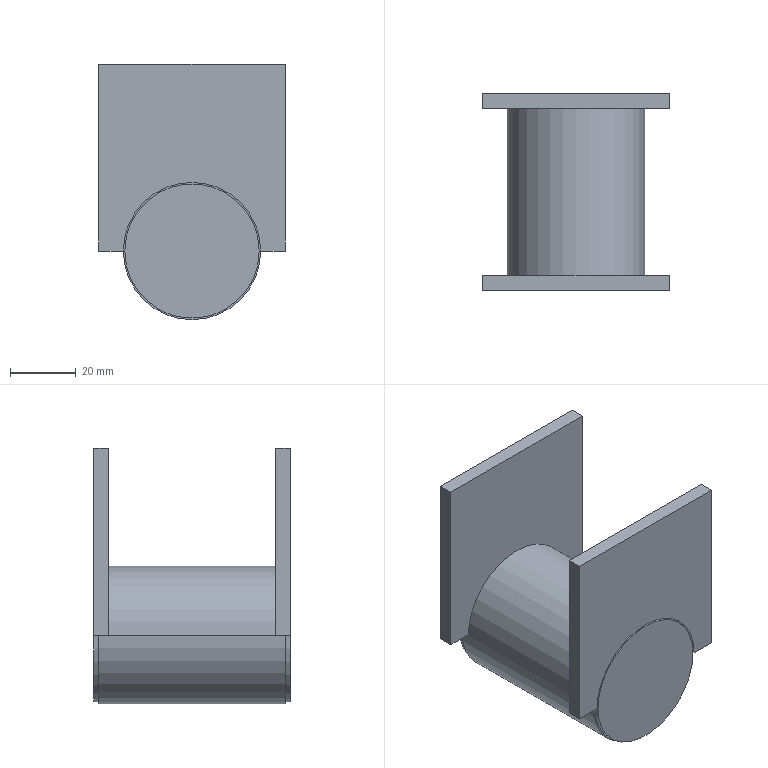Part | STEP file | 2026.6.15-Main Assembly图.sldasm-Part-221 | 1 solid | 38 faces | box 57 x 60 x 77.955 mm | volume 36451 mm3 | plane 22 | cylinder 16 | commonest cylinder face diameters 41.91 x6 41.01 x4 34.536 x2 34.968 x2 40.11 x2
STEP:
#1=CARTESIAN_POINT('',(-1591.293,1395.764,3370.147));
#2=VERTEX_POINT('',#1);
#3=CARTESIAN_POINT('',(-1591.293,1452.764,3370.147));
#4=VERTEX_POINT('',#3);
#5=CARTESIAN_POINT('',(-1591.293,1395.764,3370.147));
#6=DIRECTION('',(0.,1.,0.));
#7=VECTOR('',#6,1000.);
#8=LINE('',#5,#7);
#9=EDGE_CURVE('',#2,#4,#8,.T.);
#10=ORIENTED_EDGE('',*,*,#9,.F.);
#11=CARTESIAN_POINT('',(-1551.183,1395.764,3370.147));
#12=VERTEX_POINT('',#11);
#13=CARTESIAN_POINT('',(-1571.238,1395.764,3370.147));
#14=DIRECTION('',(0.,1.,0.));
#15=DIRECTION('',(1.,0.,0.));
#16=AXIS2_PLACEMENT_3D('',#13,#14,#15);
#17=CIRCLE('',#16,20.055);
#18=EDGE_CURVE('',#2,#12,#17,.T.);
#19=ORIENTED_EDGE('',*,*,#18,.T.);
#20=CARTESIAN_POINT('',(-1551.183,1452.764,3370.147));
#21=VERTEX_POINT('',#20);
#22=CARTESIAN_POINT('',(-1551.183,1395.764,3370.147));
#23=DIRECTION('',(0.,1.,0.));
#24=VECTOR('',#23,1000.);
#25=LINE('',#22,#24);
#26=EDGE_CURVE('',#12,#21,#25,.T.);
#27=ORIENTED_EDGE('',*,*,#26,.T.);
#28=CARTESIAN_POINT('',(-1571.238,1452.764,3370.147));
#29=DIRECTION('',(0.,-1.,0.));
#30=DIRECTION('',(1.,0.,0.));
#31=AXIS2_PLACEMENT_3D('',#28,#29,#30);
#32=CIRCLE('',#31,20.055);
#33=EDGE_CURVE('',#21,#4,#32,.T.);
#34=ORIENTED_EDGE('',*,*,#33,.T.);
#35=EDGE_LOOP('',(#10,#19,#27,#34));
#36=FACE_OUTER_BOUND('',#35,.T.);
#37=CARTESIAN_POINT('',(-1571.238,1395.764,3370.147));
#38=DIRECTION('',(0.,1.,0.));
#39=DIRECTION('',(-1.,0.,0.));
#40=AXIS2_PLACEMENT_3D('',#37,#38,#39);
#41=CYLINDRICAL_SURFACE('',#40,20.055);
#42=ADVANCED_FACE('',(#36),#41,.T.);
#43=CARTESIAN_POINT('',(-1588.506,1451.264,3370.147));
#44=VERTEX_POINT('',#43);
#45=CARTESIAN_POINT('',(-1588.506,1452.764,3370.147));
#46=VERTEX_POINT('',#45);
#47=CARTESIAN_POINT('',(-1588.506,1451.264,3370.147));
#48=DIRECTION('',(0.,1.,0.));
#49=VECTOR('',#48,1000.);
#50=LINE('',#47,#49);
#51=EDGE_CURVE('',#44,#46,#50,.T.);
#52=ORIENTED_EDGE('',*,*,#51,.F.);
#53=CARTESIAN_POINT('',(-1553.97,1451.264,3370.147));
#54=VERTEX_POINT('',#53);
#55=CARTESIAN_POINT('',(-1571.238,1451.264,3370.147));
#56=DIRECTION('',(0.,1.,0.));
#57=DIRECTION('',(1.,0.,0.));
#58=AXIS2_PLACEMENT_3D('',#55,#56,#57);
#59=CIRCLE('',#58,17.268);
#60=EDGE_CURVE('',#54,#44,#59,.T.);
#61=ORIENTED_EDGE('',*,*,#60,.F.);
#62=CARTESIAN_POINT('',(-1553.97,1452.764,3370.147));
#63=VERTEX_POINT('',#62);
#64=CARTESIAN_POINT('',(-1553.97,1451.264,3370.147));
#65=DIRECTION('',(0.,1.,0.));
#66=VECTOR('',#65,1000.);
#67=LINE('',#64,#66);
#68=EDGE_CURVE('',#54,#63,#67,.T.);
#69=ORIENTED_EDGE('',*,*,#68,.T.);
#70=CARTESIAN_POINT('',(-1571.238,1452.764,3370.147));
#71=DIRECTION('',(0.,1.,0.));
#72=DIRECTION('',(1.,0.,0.));
#73=AXIS2_PLACEMENT_3D('',#70,#71,#72);
#74=CIRCLE('',#73,17.268);
#75=EDGE_CURVE('',#63,#46,#74,.T.);
#76=ORIENTED_EDGE('',*,*,#75,.T.);
#77=EDGE_LOOP('',(#52,#61,#69,#76));
#78=FACE_OUTER_BOUND('',#77,.T.);
#79=CARTESIAN_POINT('',(-1571.238,1451.264,3370.147));
#80=DIRECTION('',(0.,1.,0.));
#81=DIRECTION('',(-1.,0.,0.));
#82=AXIS2_PLACEMENT_3D('',#79,#80,#81);
#83=CYLINDRICAL_SURFACE('',#82,17.268);
#84=ADVANCED_FACE('',(#78),#83,.F.);
#85=CARTESIAN_POINT('',(-1553.754,1395.764,3370.147));
#86=VERTEX_POINT('',#85);
#87=CARTESIAN_POINT('',(-1553.754,1397.264,3370.147));
#88=VERTEX_POINT('',#87);
#89=CARTESIAN_POINT('',(-1553.754,1397.264,3370.147));
#90=DIRECTION('',(0.,1.,0.));
#91=VECTOR('',#90,1000.);
#92=LINE('',#89,#91);
#93=EDGE_CURVE('',#86,#88,#92,.T.);
#94=ORIENTED_EDGE('',*,*,#93,.T.);
#95=CARTESIAN_POINT('',(-1588.722,1397.264,3370.147));
#96=VERTEX_POINT('',#95);
#97=CARTESIAN_POINT('',(-1571.238,1397.264,3370.147));
#98=DIRECTION('',(0.,-1.,0.));
#99=DIRECTION('',(-1.,0.,0.));
#100=AXIS2_PLACEMENT_3D('',#97,#98,#99);
#101=CIRCLE('',#100,17.484);
#102=EDGE_CURVE('',#96,#88,#101,.T.);
#103=ORIENTED_EDGE('',*,*,#102,.F.);
#104=CARTESIAN_POINT('',(-1588.722,1395.764,3370.147));
#105=VERTEX_POINT('',#104);
#106=CARTESIAN_POINT('',(-1588.722,1397.264,3370.147));
#107=DIRECTION('',(0.,1.,0.));
#108=VECTOR('',#107,1000.);
#109=LINE('',#106,#108);
#110=EDGE_CURVE('',#105,#96,#109,.T.);
#111=ORIENTED_EDGE('',*,*,#110,.F.);
#112=CARTESIAN_POINT('',(-1571.238,1395.764,3370.147));
#113=DIRECTION('',(0.,-1.,0.));
#114=DIRECTION('',(-1.,0.,0.));
#115=AXIS2_PLACEMENT_3D('',#112,#113,#114);
#116=CIRCLE('',#115,17.484);
#117=EDGE_CURVE('',#105,#86,#116,.T.);
#118=ORIENTED_EDGE('',*,*,#117,.T.);
#119=EDGE_LOOP('',(#94,#103,#111,#118));
#120=FACE_OUTER_BOUND('',#119,.T.);
#121=CARTESIAN_POINT('',(-1571.238,1397.264,3370.147));
#122=DIRECTION('',(0.,-1.,0.));
#123=DIRECTION('',(1.,0.,0.));
#124=AXIS2_PLACEMENT_3D('',#121,#122,#123);
#125=CYLINDRICAL_SURFACE('',#124,17.484);
#126=ADVANCED_FACE('',(#120),#125,.F.);
#127=CARTESIAN_POINT('',(-1571.238,1397.264,3370.147));
#128=DIRECTION('',(0.,-1.,0.));
#129=DIRECTION('',(-1.,0.,0.));
#130=AXIS2_PLACEMENT_3D('',#127,#128,#129);
#131=CIRCLE('',#130,17.484);
#132=EDGE_CURVE('',#88,#96,#131,.T.);
#133=ORIENTED_EDGE('',*,*,#132,.F.);
#134=ORIENTED_EDGE('',*,*,#93,.F.);
#135=CARTESIAN_POINT('',(-1571.238,1395.764,3370.147));
#136=DIRECTION('',(0.,-1.,0.));
#137=DIRECTION('',(-1.,0.,0.));
#138=AXIS2_PLACEMENT_3D('',#135,#136,#137);
#139=CIRCLE('',#138,17.484);
#140=EDGE_CURVE('',#86,#105,#139,.T.);
#141=ORIENTED_EDGE('',*,*,#140,.T.);
#142=ORIENTED_EDGE('',*,*,#110,.T.);
#143=EDGE_LOOP('',(#133,#134,#141,#142));
#144=FACE_OUTER_BOUND('',#143,.T.);
#145=CARTESIAN_POINT('',(-1571.238,1397.264,3370.147));
#146=DIRECTION('',(0.,-1.,0.));
#147=DIRECTION('',(1.,0.,0.));
#148=AXIS2_PLACEMENT_3D('',#145,#146,#147);
#149=CYLINDRICAL_SURFACE('',#148,17.484);
#150=ADVANCED_FACE('',(#144),#149,.F.);
#151=ORIENTED_EDGE('',*,*,#132,.T.);
#152=ORIENTED_EDGE('',*,*,#102,.T.);
#153=EDGE_LOOP('',(#151,#152));
#154=FACE_OUTER_BOUND('',#153,.T.);
#155=CARTESIAN_POINT('',(-1571.238,1397.264,3370.147));
#156=DIRECTION('',(0.,-1.,0.));
#157=DIRECTION('',(-1.,0.,0.));
#158=AXIS2_PLACEMENT_3D('',#155,#156,#157);
#159=PLANE('',#158);
#160=ADVANCED_FACE('',(#154),#159,.T.);
#161=CARTESIAN_POINT('',(-1571.238,1451.264,3370.147));
#162=DIRECTION('',(0.,1.,0.));
#163=DIRECTION('',(1.,0.,0.));
#164=AXIS2_PLACEMENT_3D('',#161,#162,#163);
#165=CIRCLE('',#164,17.268);
#166=EDGE_CURVE('',#44,#54,#165,.T.);
#167=ORIENTED_EDGE('',*,*,#166,.T.);
#168=ORIENTED_EDGE('',*,*,#60,.T.);
#169=EDGE_LOOP('',(#167,#168));
#170=FACE_OUTER_BOUND('',#169,.T.);
#171=CARTESIAN_POINT('',(-1571.238,1451.264,3370.147));
#172=DIRECTION('',(0.,1.,0.));
#173=DIRECTION('',(1.,0.,0.));
#174=AXIS2_PLACEMENT_3D('',#171,#172,#173);
#175=PLANE('',#174);
#176=ADVANCED_FACE('',(#170),#175,.T.);
#177=ORIENTED_EDGE('',*,*,#166,.F.);
#178=ORIENTED_EDGE('',*,*,#51,.T.);
#179=CARTESIAN_POINT('',(-1571.238,1452.764,3370.147));
#180=DIRECTION('',(0.,1.,0.));
#181=DIRECTION('',(1.,0.,0.));
#182=AXIS2_PLACEMENT_3D('',#179,#180,#181);
#183=CIRCLE('',#182,17.268);
#184=EDGE_CURVE('',#46,#63,#183,.T.);
#185=ORIENTED_EDGE('',*,*,#184,.T.);
#186=ORIENTED_EDGE('',*,*,#68,.F.);
#187=EDGE_LOOP('',(#177,#178,#185,#186));
#188=FACE_OUTER_BOUND('',#187,.T.);
#189=CARTESIAN_POINT('',(-1571.238,1451.264,3370.147));
#190=DIRECTION('',(0.,1.,0.));
#191=DIRECTION('',(-1.,0.,0.));
#192=AXIS2_PLACEMENT_3D('',#189,#190,#191);
#193=CYLINDRICAL_SURFACE('',#192,17.268);
#194=ADVANCED_FACE('',(#188),#193,.F.);
#195=CARTESIAN_POINT('',(-1571.238,1452.764,3370.147));
#196=DIRECTION('',(0.,-1.,0.));
#197=DIRECTION('',(1.,0.,0.));
#198=AXIS2_PLACEMENT_3D('',#195,#196,#197);
#199=CIRCLE('',#198,20.055);
#200=EDGE_CURVE('',#4,#21,#199,.T.);
#201=ORIENTED_EDGE('',*,*,#200,.F.);
#202=ORIENTED_EDGE('',*,*,#33,.F.);
#203=EDGE_LOOP('',(#201,#202));
#204=FACE_OUTER_BOUND('',#203,.T.);
#205=ORIENTED_EDGE('',*,*,#184,.F.);
#206=ORIENTED_EDGE('',*,*,#75,.F.);
#207=EDGE_LOOP('',(#205,#206));
#208=FACE_BOUND('',#207,.T.);
#209=CARTESIAN_POINT('',(-1571.238,1452.764,3370.147));
#210=DIRECTION('',(0.,1.,0.));
#211=DIRECTION('',(1.,0.,0.));
#212=AXIS2_PLACEMENT_3D('',#209,#210,#211);
#213=PLANE('',#212);
#214=ADVANCED_FACE('',(#204,#208),#213,.T.);
#215=CARTESIAN_POINT('',(-1571.238,1395.764,3370.147));
#216=DIRECTION('',(0.,1.,0.));
#217=DIRECTION('',(1.,0.,0.));
#218=AXIS2_PLACEMENT_3D('',#215,#216,#217);
#219=CIRCLE('',#218,20.055);
#220=EDGE_CURVE('',#12,#2,#219,.T.);
#221=ORIENTED_EDGE('',*,*,#220,.T.);
#222=ORIENTED_EDGE('',*,*,#9,.T.);
#223=ORIENTED_EDGE('',*,*,#200,.T.);
#224=ORIENTED_EDGE('',*,*,#26,.F.);
#225=EDGE_LOOP('',(#221,#222,#223,#224));
#226=FACE_OUTER_BOUND('',#225,.T.);
#227=CARTESIAN_POINT('',(-1571.238,1395.764,3370.147));
#228=DIRECTION('',(0.,1.,0.));
#229=DIRECTION('',(-1.,0.,0.));
#230=AXIS2_PLACEMENT_3D('',#227,#228,#229);
#231=CYLINDRICAL_SURFACE('',#230,20.055);
#232=ADVANCED_FACE('',(#226),#231,.T.);
#233=ORIENTED_EDGE('',*,*,#18,.F.);
#234=ORIENTED_EDGE('',*,*,#220,.F.);
#235=EDGE_LOOP('',(#233,#234));
#236=FACE_OUTER_BOUND('',#235,.T.);
#237=ORIENTED_EDGE('',*,*,#140,.F.);
#238=ORIENTED_EDGE('',*,*,#117,.F.);
#239=EDGE_LOOP('',(#237,#238));
#240=FACE_BOUND('',#239,.T.);
#241=CARTESIAN_POINT('',(-1571.238,1395.764,3370.147));
#242=DIRECTION('',(0.,-1.,0.));
#243=DIRECTION('',(0.,0.,-1.));
#244=AXIS2_PLACEMENT_3D('',#241,#242,#243);
#245=PLANE('',#244);
#246=ADVANCED_FACE('',(#236,#240),#245,.T.);
#247=CLOSED_SHELL('',(#42,#84,#126,#150,#160,#176,#194,#214,#232,#246));
#248=CARTESIAN_POINT('',(-1571.238,1394.264,3391.102));
#249=VERTEX_POINT('',#248);
#250=CARTESIAN_POINT('',(-1550.283,1394.264,3370.147));
#251=VERTEX_POINT('',#250);
#252=CARTESIAN_POINT('',(-1571.238,1394.264,3370.147));
#253=DIRECTION('',(0.,1.,0.));
#254=DIRECTION('',(0.,0.,-1.));
#255=AXIS2_PLACEMENT_3D('',#252,#253,#254);
#256=CIRCLE('',#255,20.955);
#257=EDGE_CURVE('',#249,#251,#256,.T.);
#258=ORIENTED_EDGE('',*,*,#257,.F.);
#259=CARTESIAN_POINT('',(-1571.238,1395.764,3391.102));
#260=VERTEX_POINT('',#259);
#261=CARTESIAN_POINT('',(-1571.238,1394.264,3391.102));
#262=DIRECTION('',(0.,1.,0.));
#263=VECTOR('',#262,1000.);
#264=LINE('',#261,#263);
#265=EDGE_CURVE('',#249,#260,#264,.T.);
#266=ORIENTED_EDGE('',*,*,#265,.T.);
#267=CARTESIAN_POINT('',(-1550.283,1395.764,3370.147));
#268=VERTEX_POINT('',#267);
#269=CARTESIAN_POINT('',(-1571.238,1395.764,3370.147));
#270=DIRECTION('',(0.,1.,0.));
#271=DIRECTION('',(1.,0.,0.));
#272=AXIS2_PLACEMENT_3D('',#269,#270,#271);
#273=CIRCLE('',#272,20.955);
#274=EDGE_CURVE('',#260,#268,#273,.T.);
#275=ORIENTED_EDGE('',*,*,#274,.T.);
#276=CARTESIAN_POINT('',(-1550.283,1394.264,3370.147));
#277=DIRECTION('',(0.,-1.,0.));
#278=VECTOR('',#277,1000.);
#279=LINE('',#276,#278);
#280=EDGE_CURVE('',#268,#251,#279,.T.);
#281=ORIENTED_EDGE('',*,*,#280,.T.);
#282=EDGE_LOOP('',(#258,#266,#275,#281));
#283=FACE_OUTER_BOUND('',#282,.T.);
#284=CARTESIAN_POINT('',(-1571.238,1394.264,3370.147));
#285=DIRECTION('',(0.,1.,0.));
#286=DIRECTION('',(0.,0.,1.));
#287=AXIS2_PLACEMENT_3D('',#284,#285,#286);
#288=CYLINDRICAL_SURFACE('',#287,20.955);
#289=ADVANCED_FACE('',(#283),#288,.F.);
#290=CARTESIAN_POINT('',(-1550.733,1394.264,3370.147));
#291=VERTEX_POINT('',#290);
#292=CARTESIAN_POINT('',(-1591.743,1394.264,3370.147));
#293=VERTEX_POINT('',#292);
#294=CARTESIAN_POINT('',(-1571.238,1394.264,3370.147));
#295=DIRECTION('',(0.,1.,0.));
#296=DIRECTION('',(1.,0.,0.));
#297=AXIS2_PLACEMENT_3D('',#294,#295,#296);
#298=CIRCLE('',#297,20.505);
#299=EDGE_CURVE('',#291,#293,#298,.T.);
#300=ORIENTED_EDGE('',*,*,#299,.T.);
#301=CARTESIAN_POINT('',(-1591.743,1395.764,3370.147));
#302=VERTEX_POINT('',#301);
#303=CARTESIAN_POINT('',(-1591.743,1394.264,3370.147));
#304=DIRECTION('',(0.,-1.,0.));
#305=VECTOR('',#304,1000.);
#306=LINE('',#303,#305);
#307=EDGE_CURVE('',#302,#293,#306,.T.);
#308=ORIENTED_EDGE('',*,*,#307,.F.);
#309=CARTESIAN_POINT('',(-1550.733,1395.764,3370.147));
#310=VERTEX_POINT('',#309);
#311=CARTESIAN_POINT('',(-1571.238,1395.764,3370.147));
#312=DIRECTION('',(0.,-1.,0.));
#313=DIRECTION('',(-1.,0.,0.));
#314=AXIS2_PLACEMENT_3D('',#311,#312,#313);
#315=CIRCLE('',#314,20.505);
#316=EDGE_CURVE('',#302,#310,#315,.T.);
#317=ORIENTED_EDGE('',*,*,#316,.T.);
#318=CARTESIAN_POINT('',(-1550.733,1394.264,3370.147));
#319=DIRECTION('',(0.,-1.,0.));
#320=VECTOR('',#319,1000.);
#321=LINE('',#318,#320);
#322=EDGE_CURVE('',#310,#291,#321,.T.);
#323=ORIENTED_EDGE('',*,*,#322,.T.);
#324=EDGE_LOOP('',(#300,#308,#317,#323));
#325=FACE_OUTER_BOUND('',#324,.T.);
#326=CARTESIAN_POINT('',(-1571.238,1394.264,3370.147));
#327=DIRECTION('',(0.,1.,0.));
#328=DIRECTION('',(-1.,0.,0.));
#329=AXIS2_PLACEMENT_3D('',#326,#327,#328);
#330=CYLINDRICAL_SURFACE('',#329,20.505);
#331=ADVANCED_FACE('',(#325),#330,.T.);
#332=CARTESIAN_POINT('',(-1550.733,1454.264,3370.147));
#333=VERTEX_POINT('',#332);
#334=CARTESIAN_POINT('',(-1591.743,1454.264,3370.147));
#335=VERTEX_POINT('',#334);
#336=CARTESIAN_POINT('',(-1571.238,1454.264,3370.147));
#337=DIRECTION('',(0.,1.,0.));
#338=DIRECTION('',(-1.,0.,0.));
#339=AXIS2_PLACEMENT_3D('',#336,#337,#338);
#340=CIRCLE('',#339,20.505);
#341=EDGE_CURVE('',#333,#335,#340,.T.);
#342=ORIENTED_EDGE('',*,*,#341,.F.);
#343=CARTESIAN_POINT('',(-1550.733,1452.764,3370.147));
#344=VERTEX_POINT('',#343);
#345=CARTESIAN_POINT('',(-1550.733,1454.264,3370.147));
#346=DIRECTION('',(0.,-1.,0.));
#347=VECTOR('',#346,1000.);
#348=LINE('',#345,#347);
#349=EDGE_CURVE('',#333,#344,#348,.T.);
#350=ORIENTED_EDGE('',*,*,#349,.T.);
#351=CARTESIAN_POINT('',(-1591.743,1452.764,3370.147));
#352=VERTEX_POINT('',#351);
#353=CARTESIAN_POINT('',(-1571.238,1452.764,3370.147));
#354=DIRECTION('',(0.,1.,0.));
#355=DIRECTION('',(-1.,0.,0.));
#356=AXIS2_PLACEMENT_3D('',#353,#354,#355);
#357=CIRCLE('',#356,20.505);
#358=EDGE_CURVE('',#344,#352,#357,.T.);
#359=ORIENTED_EDGE('',*,*,#358,.T.);
#360=CARTESIAN_POINT('',(-1591.743,1454.264,3370.147));
#361=DIRECTION('',(0.,-1.,0.));
#362=VECTOR('',#361,1000.);
#363=LINE('',#360,#362);
#364=EDGE_CURVE('',#335,#352,#363,.T.);
#365=ORIENTED_EDGE('',*,*,#364,.F.);
#366=EDGE_LOOP('',(#342,#350,#359,#365));
#367=FACE_OUTER_BOUND('',#366,.T.);
#368=CARTESIAN_POINT('',(-1571.238,1454.264,3370.147));
#369=DIRECTION('',(0.,-1.,0.));
#370=DIRECTION('',(1.,0.,0.));
#371=AXIS2_PLACEMENT_3D('',#368,#369,#370);
#372=CYLINDRICAL_SURFACE('',#371,20.505);
#373=ADVANCED_FACE('',(#367),#372,.T.);
#374=CARTESIAN_POINT('',(-1571.238,1454.264,3391.102));
#375=VERTEX_POINT('',#374);
#376=CARTESIAN_POINT('',(-1592.193,1454.264,3370.147));
#377=VERTEX_POINT('',#376);
#378=CARTESIAN_POINT('',(-1571.238,1454.264,3370.147));
#379=DIRECTION('',(0.,-1.,0.));
#380=DIRECTION('',(0.,0.,1.));
#381=AXIS2_PLACEMENT_3D('',#378,#379,#380);
#382=CIRCLE('',#381,20.955);
#383=EDGE_CURVE('',#375,#377,#382,.T.);
#384=ORIENTED_EDGE('',*,*,#383,.F.);
#385=CARTESIAN_POINT('',(-1571.238,1452.764,3391.102));
#386=VERTEX_POINT('',#385);
#387=CARTESIAN_POINT('',(-1571.238,1454.264,3391.102));
#388=DIRECTION('',(0.,-1.,0.));
#389=VECTOR('',#388,1000.);
#390=LINE('',#387,#389);
#391=EDGE_CURVE('',#375,#386,#390,.T.);
#392=ORIENTED_EDGE('',*,*,#391,.T.);
#393=CARTESIAN_POINT('',(-1592.193,1452.764,3370.147));
#394=VERTEX_POINT('',#393);
#395=CARTESIAN_POINT('',(-1571.238,1452.764,3370.147));
#396=DIRECTION('',(0.,-1.,0.));
#397=DIRECTION('',(1.,0.,0.));
#398=AXIS2_PLACEMENT_3D('',#395,#396,#397);
#399=CIRCLE('',#398,20.955);
#400=EDGE_CURVE('',#386,#394,#399,.T.);
#401=ORIENTED_EDGE('',*,*,#400,.T.);
#402=CARTESIAN_POINT('',(-1592.193,1454.264,3370.147));
#403=DIRECTION('',(0.,1.,0.));
#404=VECTOR('',#403,1000.);
#405=LINE('',#402,#404);
#406=EDGE_CURVE('',#394,#377,#405,.T.);
#407=ORIENTED_EDGE('',*,*,#406,.T.);
#408=EDGE_LOOP('',(#384,#392,#401,#407));
#409=FACE_OUTER_BOUND('',#408,.T.);
#410=CARTESIAN_POINT('',(-1571.238,1454.264,3370.147));
#411=DIRECTION('',(0.,-1.,0.));
#412=DIRECTION('',(0.,0.,-1.));
#413=AXIS2_PLACEMENT_3D('',#410,#411,#412);
#414=CYLINDRICAL_SURFACE('',#413,20.955);
#415=ADVANCED_FACE('',(#409),#414,.F.);
#416=CARTESIAN_POINT('',(-1592.193,1398.764,3370.147));
#417=VERTEX_POINT('',#416);
#418=CARTESIAN_POINT('',(-1592.193,1395.764,3370.147));
#419=VERTEX_POINT('',#418);
#420=CARTESIAN_POINT('',(-1592.193,1394.264,3370.147));
#421=DIRECTION('',(0.,-1.,0.));
#422=VECTOR('',#421,1000.);
#423=LINE('',#420,#422);
#424=EDGE_CURVE('',#417,#419,#423,.T.);
#425=ORIENTED_EDGE('',*,*,#424,.F.);
#426=CARTESIAN_POINT('',(-1592.193,1449.764,3370.147));
#427=VERTEX_POINT('',#426);
#428=CARTESIAN_POINT('',(-1592.193,1395.764,3370.147));
#429=DIRECTION('',(0.,-1.,0.));
#430=VECTOR('',#429,1000.);
#431=LINE('',#428,#430);
#432=EDGE_CURVE('',#427,#417,#431,.T.);
#433=ORIENTED_EDGE('',*,*,#432,.F.);
#434=CARTESIAN_POINT('',(-1592.193,1454.264,3370.147));
#435=DIRECTION('',(0.,1.,0.));
#436=VECTOR('',#435,1000.);
#437=LINE('',#434,#436);
#438=EDGE_CURVE('',#427,#394,#437,.T.);
#439=ORIENTED_EDGE('',*,*,#438,.T.);
#440=CARTESIAN_POINT('',(-1550.283,1452.764,3370.147));
#441=VERTEX_POINT('',#440);
#442=CARTESIAN_POINT('',(-1571.238,1452.764,3370.147));
#443=DIRECTION('',(0.,-1.,0.));
#444=DIRECTION('',(1.,0.,0.));
#445=AXIS2_PLACEMENT_3D('',#442,#443,#444);
#446=CIRCLE('',#445,20.955);
#447=EDGE_CURVE('',#394,#441,#446,.T.);
#448=ORIENTED_EDGE('',*,*,#447,.T.);
#449=CARTESIAN_POINT('',(-1550.283,1449.764,3370.147));
#450=VERTEX_POINT('',#449);
#451=CARTESIAN_POINT('',(-1550.283,1454.264,3370.147));
#452=DIRECTION('',(0.,1.,0.));
#453=VECTOR('',#452,1000.);
#454=LINE('',#451,#453);
#455=EDGE_CURVE('',#450,#441,#454,.T.);
#456=ORIENTED_EDGE('',*,*,#455,.F.);
#457=CARTESIAN_POINT('',(-1550.283,1398.764,3370.147));
#458=VERTEX_POINT('',#457);
#459=CARTESIAN_POINT('',(-1550.283,1395.764,3370.147));
#460=DIRECTION('',(0.,-1.,0.));
#461=VECTOR('',#460,1000.);
#462=LINE('',#459,#461);
#463=EDGE_CURVE('',#450,#458,#462,.T.);
#464=ORIENTED_EDGE('',*,*,#463,.T.);
#465=CARTESIAN_POINT('',(-1550.283,1394.264,3370.147));
#466=DIRECTION('',(0.,-1.,0.));
#467=VECTOR('',#466,1000.);
#468=LINE('',#465,#467);
#469=EDGE_CURVE('',#458,#268,#468,.T.);
#470=ORIENTED_EDGE('',*,*,#469,.T.);
#471=CARTESIAN_POINT('',(-1571.238,1395.764,3370.147));
#472=DIRECTION('',(0.,1.,0.));
#473=DIRECTION('',(1.,0.,0.));
#474=AXIS2_PLACEMENT_3D('',#471,#472,#473);
#475=CIRCLE('',#474,20.955);
#476=EDGE_CURVE('',#268,#419,#475,.T.);
#477=ORIENTED_EDGE('',*,*,#476,.T.);
#478=EDGE_LOOP('',(#425,#433,#439,#448,#456,#464,#470,#477));
#479=FACE_OUTER_BOUND('',#478,.T.);
#480=CARTESIAN_POINT('',(-1571.238,1395.764,3370.147));
#481=DIRECTION('',(0.,1.,0.));
#482=DIRECTION('',(-1.,0.,0.));
#483=AXIS2_PLACEMENT_3D('',#480,#481,#482);
#484=CYLINDRICAL_SURFACE('',#483,20.955);
#485=ADVANCED_FACE('',(#479),#484,.T.);
#486=CARTESIAN_POINT('',(-1542.738,1398.764,3370.147));
#487=VERTEX_POINT('',#486);
#488=CARTESIAN_POINT('',(-1542.738,1398.764,3370.147));
#489=DIRECTION('',(-1.,0.,0.));
#490=VECTOR('',#489,1000.);
#491=LINE('',#488,#490);
#492=EDGE_CURVE('',#487,#458,#491,.T.);
#493=ORIENTED_EDGE('',*,*,#492,.T.);
#494=CARTESIAN_POINT('',(-1571.238,1398.764,3370.147));
#495=DIRECTION('',(0.,-1.,0.));
#496=DIRECTION('',(0.,0.,-1.));
#497=AXIS2_PLACEMENT_3D('',#494,#495,#496);
#498=CIRCLE('',#497,20.955);
#499=EDGE_CURVE('',#458,#417,#498,.T.);
#500=ORIENTED_EDGE('',*,*,#499,.T.);
#501=CARTESIAN_POINT('',(-1599.738,1398.764,3370.147));
#502=VERTEX_POINT('',#501);
#503=CARTESIAN_POINT('',(-1592.193,1398.764,3370.147));
#504=DIRECTION('',(-1.,0.,0.));
#505=VECTOR('',#504,1000.);
#506=LINE('',#503,#505);
#507=EDGE_CURVE('',#417,#502,#506,.T.);
#508=ORIENTED_EDGE('',*,*,#507,.T.);
#509=CARTESIAN_POINT('',(-1599.738,1398.764,3427.147));
#510=VERTEX_POINT('',#509);
#511=CARTESIAN_POINT('',(-1599.738,1398.764,3427.147));
#512=DIRECTION('',(0.,0.,1.));
#513=VECTOR('',#512,1000.);
#514=LINE('',#511,#513);
#515=EDGE_CURVE('',#502,#510,#514,.T.);
#516=ORIENTED_EDGE('',*,*,#515,.T.);
#517=CARTESIAN_POINT('',(-1542.738,1398.764,3427.147));
#518=VERTEX_POINT('',#517);
#519=CARTESIAN_POINT('',(-1542.738,1398.764,3427.147));
#520=DIRECTION('',(1.,0.,0.));
#521=VECTOR('',#520,1000.);
#522=LINE('',#519,#521);
#523=EDGE_CURVE('',#510,#518,#522,.T.);
#524=ORIENTED_EDGE('',*,*,#523,.T.);
#525=CARTESIAN_POINT('',(-1542.738,1398.764,3427.147));
#526=DIRECTION('',(0.,0.,-1.));
#527=VECTOR('',#526,1000.);
#528=LINE('',#525,#527);
#529=EDGE_CURVE('',#518,#487,#528,.T.);
#530=ORIENTED_EDGE('',*,*,#529,.T.);
#531=EDGE_LOOP('',(#493,#500,#508,#516,#524,#530));
#532=FACE_OUTER_BOUND('',#531,.T.);
#533=CARTESIAN_POINT('',(-1571.238,1398.764,3370.147));
#534=DIRECTION('',(0.,-1.,0.));
#535=DIRECTION('',(-1.,0.,0.));
#536=AXIS2_PLACEMENT_3D('',#533,#534,#535);
#537=PLANE('',#536);
#538=ADVANCED_FACE('',(#532),#537,.F.);
#539=CARTESIAN_POINT('',(-1542.738,1394.264,3427.147));
#540=VERTEX_POINT('',#539);
#541=CARTESIAN_POINT('',(-1542.738,1394.264,3427.147));
#542=DIRECTION('',(0.,-1.,0.));
#543=VECTOR('',#542,1000.);
#544=LINE('',#541,#543);
#545=EDGE_CURVE('',#518,#540,#544,.T.);
#546=ORIENTED_EDGE('',*,*,#545,.T.);
#547=CARTESIAN_POINT('',(-1542.738,1394.264,3370.147));
#548=VERTEX_POINT('',#547);
#549=CARTESIAN_POINT('',(-1542.738,1394.264,3370.147));
#550=DIRECTION('',(0.,0.,1.));
#551=VECTOR('',#550,1000.);
#552=LINE('',#549,#551);
#553=EDGE_CURVE('',#548,#540,#552,.T.);
#554=ORIENTED_EDGE('',*,*,#553,.F.);
#555=CARTESIAN_POINT('',(-1542.738,1394.264,3370.147));
#556=DIRECTION('',(0.,1.,0.));
#557=VECTOR('',#556,1000.);
#558=LINE('',#555,#557);
#559=EDGE_CURVE('',#548,#487,#558,.T.);
#560=ORIENTED_EDGE('',*,*,#559,.T.);
#561=ORIENTED_EDGE('',*,*,#529,.F.);
#562=EDGE_LOOP('',(#546,#554,#560,#561));
#563=FACE_OUTER_BOUND('',#562,.T.);
#564=CARTESIAN_POINT('',(-1542.738,1394.264,3427.147));
#565=DIRECTION('',(-1.,0.,0.));
#566=DIRECTION('',(0.,-1.,0.));
#567=AXIS2_PLACEMENT_3D('',#564,#565,#566);
#568=PLANE('',#567);
#569=ADVANCED_FACE('',(#563),#568,.F.);
#570=CARTESIAN_POINT('',(-1599.738,1394.264,3427.147));
#571=VERTEX_POINT('',#570);
#572=CARTESIAN_POINT('',(-1599.738,1394.264,3427.147));
#573=DIRECTION('',(0.,-1.,0.));
#574=VECTOR('',#573,1000.);
#575=LINE('',#572,#574);
#576=EDGE_CURVE('',#510,#571,#575,.T.);
#577=ORIENTED_EDGE('',*,*,#576,.T.);
#578=CARTESIAN_POINT('',(-1571.238,1394.264,3427.147));
#579=DIRECTION('',(-1.,0.,0.));
#580=VECTOR('',#579,1000.);
#581=LINE('',#578,#580);
#582=EDGE_CURVE('',#540,#571,#581,.T.);
#583=ORIENTED_EDGE('',*,*,#582,.F.);
#584=ORIENTED_EDGE('',*,*,#545,.F.);
#585=ORIENTED_EDGE('',*,*,#523,.F.);
#586=EDGE_LOOP('',(#577,#583,#584,#585));
#587=FACE_OUTER_BOUND('',#586,.T.);
#588=CARTESIAN_POINT('',(-1542.738,1394.264,3427.147));
#589=DIRECTION('',(0.,0.,-1.));
#590=DIRECTION('',(1.,0.,0.));
#591=AXIS2_PLACEMENT_3D('',#588,#589,#590);
#592=PLANE('',#591);
#593=ADVANCED_FACE('',(#587),#592,.F.);
#594=CARTESIAN_POINT('',(-1599.738,1394.264,3370.147));
#595=VERTEX_POINT('',#594);
#596=CARTESIAN_POINT('',(-1599.738,1394.264,3370.147));
#597=DIRECTION('',(0.,-1.,0.));
#598=VECTOR('',#597,1000.);
#599=LINE('',#596,#598);
#600=EDGE_CURVE('',#502,#595,#599,.T.);
#601=ORIENTED_EDGE('',*,*,#600,.T.);
#602=CARTESIAN_POINT('',(-1599.738,1394.264,3370.147));
#603=DIRECTION('',(0.,0.,-1.));
#604=VECTOR('',#603,1000.);
#605=LINE('',#602,#604);
#606=EDGE_CURVE('',#571,#595,#605,.T.);
#607=ORIENTED_EDGE('',*,*,#606,.F.);
#608=ORIENTED_EDGE('',*,*,#576,.F.);
#609=ORIENTED_EDGE('',*,*,#515,.F.);
#610=EDGE_LOOP('',(#601,#607,#608,#609));
#611=FACE_OUTER_BOUND('',#610,.T.);
#612=CARTESIAN_POINT('',(-1599.738,1394.264,3427.147));
#613=DIRECTION('',(1.,0.,0.));
#614=DIRECTION('',(0.,-1.,0.));
#615=AXIS2_PLACEMENT_3D('',#612,#613,#614);
#616=PLANE('',#615);
#617=ADVANCED_FACE('',(#611),#616,.F.);
#618=ORIENTED_EDGE('',*,*,#424,.T.);
#619=CARTESIAN_POINT('',(-1592.193,1394.264,3370.147));
#620=VERTEX_POINT('',#619);
#621=CARTESIAN_POINT('',(-1592.193,1394.264,3370.147));
#622=DIRECTION('',(0.,-1.,0.));
#623=VECTOR('',#622,1000.);
#624=LINE('',#621,#623);
#625=EDGE_CURVE('',#419,#620,#624,.T.);
#626=ORIENTED_EDGE('',*,*,#625,.T.);
#627=CARTESIAN_POINT('',(-1571.238,1394.264,3370.147));
#628=DIRECTION('',(1.,0.,0.));
#629=VECTOR('',#628,1000.);
#630=LINE('',#627,#629);
#631=EDGE_CURVE('',#595,#620,#630,.T.);
#632=ORIENTED_EDGE('',*,*,#631,.F.);
#633=ORIENTED_EDGE('',*,*,#600,.F.);
#634=ORIENTED_EDGE('',*,*,#507,.F.);
#635=EDGE_LOOP('',(#618,#626,#632,#633,#634));
#636=FACE_OUTER_BOUND('',#635,.T.);
#637=CARTESIAN_POINT('',(-1592.193,1394.264,3370.147));
#638=DIRECTION('',(0.,0.,1.));
#639=DIRECTION('',(-1.,0.,0.));
#640=AXIS2_PLACEMENT_3D('',#637,#638,#639);
#641=PLANE('',#640);
#642=ADVANCED_FACE('',(#636),#641,.F.);
#643=ORIENTED_EDGE('',*,*,#265,.F.);
#644=CARTESIAN_POINT('',(-1571.238,1394.264,3370.147));
#645=DIRECTION('',(0.,1.,0.));
#646=DIRECTION('',(0.,0.,-1.));
#647=AXIS2_PLACEMENT_3D('',#644,#645,#646);
#648=CIRCLE('',#647,20.955);
#649=EDGE_CURVE('',#620,#249,#648,.T.);
#650=ORIENTED_EDGE('',*,*,#649,.F.);
#651=ORIENTED_EDGE('',*,*,#625,.F.);
#652=CARTESIAN_POINT('',(-1571.238,1395.764,3370.147));
#653=DIRECTION('',(0.,1.,0.));
#654=DIRECTION('',(1.,0.,0.));
#655=AXIS2_PLACEMENT_3D('',#652,#653,#654);
#656=CIRCLE('',#655,20.955);
#657=EDGE_CURVE('',#419,#260,#656,.T.);
#658=ORIENTED_EDGE('',*,*,#657,.T.);
#659=EDGE_LOOP('',(#643,#650,#651,#658));
#660=FACE_OUTER_BOUND('',#659,.T.);
#661=CARTESIAN_POINT('',(-1571.238,1394.264,3370.147));
#662=DIRECTION('',(0.,1.,0.));
#663=DIRECTION('',(0.,0.,1.));
#664=AXIS2_PLACEMENT_3D('',#661,#662,#663);
#665=CYLINDRICAL_SURFACE('',#664,20.955);
#666=ADVANCED_FACE('',(#660),#665,.F.);
#667=ORIENTED_EDGE('',*,*,#559,.F.);
#668=CARTESIAN_POINT('',(-1571.238,1394.264,3370.147));
#669=DIRECTION('',(1.,0.,0.));
#670=VECTOR('',#669,1000.);
#671=LINE('',#668,#670);
#672=EDGE_CURVE('',#251,#548,#671,.T.);
#673=ORIENTED_EDGE('',*,*,#672,.F.);
#674=ORIENTED_EDGE('',*,*,#280,.F.);
#675=ORIENTED_EDGE('',*,*,#469,.F.);
#676=ORIENTED_EDGE('',*,*,#492,.F.);
#677=EDGE_LOOP('',(#667,#673,#674,#675,#676));
#678=FACE_OUTER_BOUND('',#677,.T.);
#679=CARTESIAN_POINT('',(-1542.738,1394.264,3370.147));
#680=DIRECTION('',(0.,0.,1.));
#681=DIRECTION('',(-1.,0.,0.));
#682=AXIS2_PLACEMENT_3D('',#679,#680,#681);
#683=PLANE('',#682);
#684=ADVANCED_FACE('',(#678),#683,.F.);
#685=ORIENTED_EDGE('',*,*,#649,.T.);
#686=ORIENTED_EDGE('',*,*,#257,.T.);
#687=ORIENTED_EDGE('',*,*,#672,.T.);
#688=ORIENTED_EDGE('',*,*,#553,.T.);
#689=ORIENTED_EDGE('',*,*,#582,.T.);
#690=ORIENTED_EDGE('',*,*,#606,.T.);
#691=ORIENTED_EDGE('',*,*,#631,.T.);
#692=EDGE_LOOP('',(#685,#686,#687,#688,#689,#690,#691));
#693=FACE_OUTER_BOUND('',#692,.T.);
#694=CARTESIAN_POINT('',(-1571.238,1394.264,3370.147));
#695=DIRECTION('',(0.,-1.,0.));
#696=DIRECTION('',(-1.,0.,0.));
#697=AXIS2_PLACEMENT_3D('',#694,#695,#696);
#698=PLANE('',#697);
#699=ADVANCED_FACE('',(#693),#698,.T.);
#700=ORIENTED_EDGE('',*,*,#432,.T.);
#701=ORIENTED_EDGE('',*,*,#499,.F.);
#702=ORIENTED_EDGE('',*,*,#463,.F.);
#703=CARTESIAN_POINT('',(-1571.238,1449.764,3370.147));
#704=DIRECTION('',(0.,1.,0.));
#705=DIRECTION('',(0.,0.,1.));
#706=AXIS2_PLACEMENT_3D('',#703,#704,#705);
#707=CIRCLE('',#706,20.955);
#708=EDGE_CURVE('',#427,#450,#707,.T.);
#709=ORIENTED_EDGE('',*,*,#708,.F.);
#710=EDGE_LOOP('',(#700,#701,#702,#709));
#711=FACE_OUTER_BOUND('',#710,.T.);
#712=CARTESIAN_POINT('',(-1571.238,1395.764,3370.147));
#713=DIRECTION('',(0.,1.,0.));
#714=DIRECTION('',(-1.,0.,0.));
#715=AXIS2_PLACEMENT_3D('',#712,#713,#714);
#716=CYLINDRICAL_SURFACE('',#715,20.955);
#717=ADVANCED_FACE('',(#711),#716,.T.);
#718=ORIENTED_EDGE('',*,*,#391,.F.);
#719=CARTESIAN_POINT('',(-1550.283,1454.264,3370.147));
#720=VERTEX_POINT('',#719);
#721=CARTESIAN_POINT('',(-1571.238,1454.264,3370.147));
#722=DIRECTION('',(0.,-1.,0.));
#723=DIRECTION('',(0.,0.,1.));
#724=AXIS2_PLACEMENT_3D('',#721,#722,#723);
#725=CIRCLE('',#724,20.955);
#726=EDGE_CURVE('',#720,#375,#725,.T.);
#727=ORIENTED_EDGE('',*,*,#726,.F.);
#728=CARTESIAN_POINT('',(-1550.283,1454.264,3370.147));
#729=DIRECTION('',(0.,1.,0.));
#730=VECTOR('',#729,1000.);
#731=LINE('',#728,#730);
#732=EDGE_CURVE('',#441,#720,#731,.T.);
#733=ORIENTED_EDGE('',*,*,#732,.F.);
#734=CARTESIAN_POINT('',(-1571.238,1452.764,3370.147));
#735=DIRECTION('',(0.,-1.,0.));
#736=DIRECTION('',(1.,0.,0.));
#737=AXIS2_PLACEMENT_3D('',#734,#735,#736);
#738=CIRCLE('',#737,20.955);
#739=EDGE_CURVE('',#441,#386,#738,.T.);
#740=ORIENTED_EDGE('',*,*,#739,.T.);
#741=EDGE_LOOP('',(#718,#727,#733,#740));
#742=FACE_OUTER_BOUND('',#741,.T.);
#743=CARTESIAN_POINT('',(-1571.238,1454.264,3370.147));
#744=DIRECTION('',(0.,-1.,0.));
#745=DIRECTION('',(0.,0.,-1.));
#746=AXIS2_PLACEMENT_3D('',#743,#744,#745);
#747=CYLINDRICAL_SURFACE('',#746,20.955);
#748=ADVANCED_FACE('',(#742),#747,.F.);
#749=CARTESIAN_POINT('',(-1599.738,1449.764,3427.147));
#750=VERTEX_POINT('',#749);
#751=CARTESIAN_POINT('',(-1599.738,1449.764,3370.147));
#752=VERTEX_POINT('',#751);
#753=CARTESIAN_POINT('',(-1599.738,1449.764,3370.147));
#754=DIRECTION('',(0.,0.,-1.));
#755=VECTOR('',#754,1000.);
#756=LINE('',#753,#755);
#757=EDGE_CURVE('',#750,#752,#756,.T.);
#758=ORIENTED_EDGE('',*,*,#757,.T.);
#759=CARTESIAN_POINT('',(-1592.193,1449.764,3370.147));
#760=DIRECTION('',(1.,0.,0.));
#761=VECTOR('',#760,1000.);
#762=LINE('',#759,#761);
#763=EDGE_CURVE('',#752,#427,#762,.T.);
#764=ORIENTED_EDGE('',*,*,#763,.T.);
#765=ORIENTED_EDGE('',*,*,#708,.T.);
#766=CARTESIAN_POINT('',(-1542.738,1449.764,3370.147));
#767=VERTEX_POINT('',#766);
#768=CARTESIAN_POINT('',(-1542.738,1449.764,3370.147));
#769=DIRECTION('',(1.,0.,0.));
#770=VECTOR('',#769,1000.);
#771=LINE('',#768,#770);
#772=EDGE_CURVE('',#450,#767,#771,.T.);
#773=ORIENTED_EDGE('',*,*,#772,.T.);
#774=CARTESIAN_POINT('',(-1542.738,1449.764,3427.147));
#775=VERTEX_POINT('',#774);
#776=CARTESIAN_POINT('',(-1542.738,1449.764,3427.147));
#777=DIRECTION('',(0.,0.,1.));
#778=VECTOR('',#777,1000.);
#779=LINE('',#776,#778);
#780=EDGE_CURVE('',#767,#775,#779,.T.);
#781=ORIENTED_EDGE('',*,*,#780,.T.);
#782=CARTESIAN_POINT('',(-1599.738,1449.764,3427.147));
#783=DIRECTION('',(-1.,0.,0.));
#784=VECTOR('',#783,1000.);
#785=LINE('',#782,#784);
#786=EDGE_CURVE('',#775,#750,#785,.T.);
#787=ORIENTED_EDGE('',*,*,#786,.T.);
#788=EDGE_LOOP('',(#758,#764,#765,#773,#781,#787));
#789=FACE_OUTER_BOUND('',#788,.T.);
#790=CARTESIAN_POINT('',(-1571.238,1449.764,3370.147));
#791=DIRECTION('',(0.,1.,0.));
#792=DIRECTION('',(1.,0.,0.));
#793=AXIS2_PLACEMENT_3D('',#790,#791,#792);
#794=PLANE('',#793);
#795=ADVANCED_FACE('',(#789),#794,.F.);
#796=CARTESIAN_POINT('',(-1542.738,1454.264,3427.147));
#797=VERTEX_POINT('',#796);
#798=CARTESIAN_POINT('',(-1542.738,1454.264,3427.147));
#799=DIRECTION('',(0.,1.,0.));
#800=VECTOR('',#799,1000.);
#801=LINE('',#798,#800);
#802=EDGE_CURVE('',#775,#797,#801,.T.);
#803=ORIENTED_EDGE('',*,*,#802,.T.);
#804=CARTESIAN_POINT('',(-1599.738,1454.264,3427.147));
#805=VERTEX_POINT('',#804);
#806=CARTESIAN_POINT('',(-1571.238,1454.264,3427.147));
#807=DIRECTION('',(1.,0.,0.));
#808=VECTOR('',#807,1000.);
#809=LINE('',#806,#808);
#810=EDGE_CURVE('',#805,#797,#809,.T.);
#811=ORIENTED_EDGE('',*,*,#810,.F.);
#812=CARTESIAN_POINT('',(-1599.738,1454.264,3427.147));
#813=DIRECTION('',(0.,-1.,0.));
#814=VECTOR('',#813,1000.);
#815=LINE('',#812,#814);
#816=EDGE_CURVE('',#805,#750,#815,.T.);
#817=ORIENTED_EDGE('',*,*,#816,.T.);
#818=ORIENTED_EDGE('',*,*,#786,.F.);
#819=EDGE_LOOP('',(#803,#811,#817,#818));
#820=FACE_OUTER_BOUND('',#819,.T.);
#821=CARTESIAN_POINT('',(-1599.738,1454.264,3427.147));
#822=DIRECTION('',(0.,0.,-1.));
#823=DIRECTION('',(1.,0.,0.));
#824=AXIS2_PLACEMENT_3D('',#821,#822,#823);
#825=PLANE('',#824);
#826=ADVANCED_FACE('',(#820),#825,.F.);
#827=CARTESIAN_POINT('',(-1542.738,1454.264,3370.147));
#828=VERTEX_POINT('',#827);
#829=CARTESIAN_POINT('',(-1542.738,1454.264,3370.147));
#830=DIRECTION('',(0.,1.,0.));
#831=VECTOR('',#830,1000.);
#832=LINE('',#829,#831);
#833=EDGE_CURVE('',#767,#828,#832,.T.);
#834=ORIENTED_EDGE('',*,*,#833,.T.);
#835=CARTESIAN_POINT('',(-1542.738,1454.264,3370.147));
#836=DIRECTION('',(0.,0.,-1.));
#837=VECTOR('',#836,1000.);
#838=LINE('',#835,#837);
#839=EDGE_CURVE('',#797,#828,#838,.T.);
#840=ORIENTED_EDGE('',*,*,#839,.F.);
#841=ORIENTED_EDGE('',*,*,#802,.F.);
#842=ORIENTED_EDGE('',*,*,#780,.F.);
#843=EDGE_LOOP('',(#834,#840,#841,#842));
#844=FACE_OUTER_BOUND('',#843,.T.);
#845=CARTESIAN_POINT('',(-1542.738,1454.264,3427.147));
#846=DIRECTION('',(-1.,0.,0.));
#847=DIRECTION('',(0.,-1.,0.));
#848=AXIS2_PLACEMENT_3D('',#845,#846,#847);
#849=PLANE('',#848);
#850=ADVANCED_FACE('',(#844),#849,.F.);
#851=ORIENTED_EDGE('',*,*,#455,.T.);
#852=ORIENTED_EDGE('',*,*,#732,.T.);
#853=CARTESIAN_POINT('',(-1571.238,1454.264,3370.147));
#854=DIRECTION('',(-1.,0.,0.));
#855=VECTOR('',#854,1000.);
#856=LINE('',#853,#855);
#857=EDGE_CURVE('',#828,#720,#856,.T.);
#858=ORIENTED_EDGE('',*,*,#857,.F.);
#859=ORIENTED_EDGE('',*,*,#833,.F.);
#860=ORIENTED_EDGE('',*,*,#772,.F.);
#861=EDGE_LOOP('',(#851,#852,#858,#859,#860));
#862=FACE_OUTER_BOUND('',#861,.T.);
#863=CARTESIAN_POINT('',(-1542.738,1454.264,3370.147));
#864=DIRECTION('',(0.,0.,1.));
#865=DIRECTION('',(0.,1.,0.));
#866=AXIS2_PLACEMENT_3D('',#863,#864,#865);
#867=PLANE('',#866);
#868=ADVANCED_FACE('',(#862),#867,.F.);
#869=CARTESIAN_POINT('',(-1599.738,1454.264,3370.147));
#870=VERTEX_POINT('',#869);
#871=CARTESIAN_POINT('',(-1599.738,1454.264,3370.147));
#872=DIRECTION('',(0.,1.,0.));
#873=VECTOR('',#872,1000.);
#874=LINE('',#871,#873);
#875=EDGE_CURVE('',#752,#870,#874,.T.);
#876=ORIENTED_EDGE('',*,*,#875,.T.);
#877=CARTESIAN_POINT('',(-1571.238,1454.264,3370.147));
#878=DIRECTION('',(-1.,0.,0.));
#879=VECTOR('',#878,1000.);
#880=LINE('',#877,#879);
#881=EDGE_CURVE('',#377,#870,#880,.T.);
#882=ORIENTED_EDGE('',*,*,#881,.F.);
#883=ORIENTED_EDGE('',*,*,#406,.F.);
#884=ORIENTED_EDGE('',*,*,#438,.F.);
#885=ORIENTED_EDGE('',*,*,#763,.F.);
#886=EDGE_LOOP('',(#876,#882,#883,#884,#885));
#887=FACE_OUTER_BOUND('',#886,.T.);
#888=CARTESIAN_POINT('',(-1592.193,1454.264,3370.147));
#889=DIRECTION('',(0.,0.,1.));
#890=DIRECTION('',(-1.,0.,0.));
#891=AXIS2_PLACEMENT_3D('',#888,#889,#890);
#892=PLANE('',#891);
#893=ADVANCED_FACE('',(#887),#892,.F.);
#894=ORIENTED_EDGE('',*,*,#816,.F.);
#895=CARTESIAN_POINT('',(-1599.738,1454.264,3370.147));
#896=DIRECTION('',(0.,0.,1.));
#897=VECTOR('',#896,1000.);
#898=LINE('',#895,#897);
#899=EDGE_CURVE('',#870,#805,#898,.T.);
#900=ORIENTED_EDGE('',*,*,#899,.F.);
#901=ORIENTED_EDGE('',*,*,#875,.F.);
#902=ORIENTED_EDGE('',*,*,#757,.F.);
#903=EDGE_LOOP('',(#894,#900,#901,#902));
#904=FACE_OUTER_BOUND('',#903,.T.);
#905=CARTESIAN_POINT('',(-1599.738,1454.264,3370.147));
#906=DIRECTION('',(1.,0.,0.));
#907=DIRECTION('',(0.,-1.,0.));
#908=AXIS2_PLACEMENT_3D('',#905,#906,#907);
#909=PLANE('',#908);
#910=ADVANCED_FACE('',(#904),#909,.F.);
#911=ORIENTED_EDGE('',*,*,#881,.T.);
#912=ORIENTED_EDGE('',*,*,#899,.T.);
#913=ORIENTED_EDGE('',*,*,#810,.T.);
#914=ORIENTED_EDGE('',*,*,#839,.T.);
#915=ORIENTED_EDGE('',*,*,#857,.T.);
#916=ORIENTED_EDGE('',*,*,#726,.T.);
#917=ORIENTED_EDGE('',*,*,#383,.T.);
#918=EDGE_LOOP('',(#911,#912,#913,#914,#915,#916,#917));
#919=FACE_OUTER_BOUND('',#918,.T.);
#920=CARTESIAN_POINT('',(-1571.238,1454.264,3370.147));
#921=DIRECTION('',(0.,1.,0.));
#922=DIRECTION('',(1.,0.,0.));
#923=AXIS2_PLACEMENT_3D('',#920,#921,#922);
#924=PLANE('',#923);
#925=ADVANCED_FACE('',(#919),#924,.T.);
#926=ORIENTED_EDGE('',*,*,#476,.F.);
#927=ORIENTED_EDGE('',*,*,#274,.F.);
#928=ORIENTED_EDGE('',*,*,#657,.F.);
#929=EDGE_LOOP('',(#926,#927,#928));
#930=FACE_OUTER_BOUND('',#929,.T.);
#931=CARTESIAN_POINT('',(-1571.238,1395.764,3370.147));
#932=DIRECTION('',(0.,-1.,0.));
#933=DIRECTION('',(-1.,0.,0.));
#934=AXIS2_PLACEMENT_3D('',#931,#932,#933);
#935=CIRCLE('',#934,20.505);
#936=EDGE_CURVE('',#310,#302,#935,.T.);
#937=ORIENTED_EDGE('',*,*,#936,.F.);
#938=ORIENTED_EDGE('',*,*,#316,.F.);
#939=EDGE_LOOP('',(#937,#938));
#940=FACE_BOUND('',#939,.T.);
#941=CARTESIAN_POINT('',(-1571.238,1395.764,3370.147));
#942=DIRECTION('',(0.,-1.,0.));
#943=DIRECTION('',(0.,0.,-1.));
#944=AXIS2_PLACEMENT_3D('',#941,#942,#943);
#945=PLANE('',#944);
#946=ADVANCED_FACE('',(#930,#940),#945,.T.);
#947=ORIENTED_EDGE('',*,*,#739,.F.);
#948=ORIENTED_EDGE('',*,*,#447,.F.);
#949=ORIENTED_EDGE('',*,*,#400,.F.);
#950=EDGE_LOOP('',(#947,#948,#949));
#951=FACE_OUTER_BOUND('',#950,.T.);
#952=CARTESIAN_POINT('',(-1571.238,1452.764,3370.147));
#953=DIRECTION('',(0.,1.,0.));
#954=DIRECTION('',(-1.,0.,0.));
#955=AXIS2_PLACEMENT_3D('',#952,#953,#954);
#956=CIRCLE('',#955,20.505);
#957=EDGE_CURVE('',#352,#344,#956,.T.);
#958=ORIENTED_EDGE('',*,*,#957,.F.);
#959=ORIENTED_EDGE('',*,*,#358,.F.);
#960=EDGE_LOOP('',(#958,#959));
#961=FACE_BOUND('',#960,.T.);
#962=CARTESIAN_POINT('',(-1571.238,1452.764,3370.147));
#963=DIRECTION('',(0.,-1.,0.));
#964=DIRECTION('',(0.,0.,-1.));
#965=AXIS2_PLACEMENT_3D('',#962,#963,#964);
#966=PLANE('',#965);
#967=ADVANCED_FACE('',(#951,#961),#966,.F.);
#968=ORIENTED_EDGE('',*,*,#349,.F.);
#969=CARTESIAN_POINT('',(-1571.238,1454.264,3370.147));
#970=DIRECTION('',(0.,1.,0.));
#971=DIRECTION('',(-1.,0.,0.));
#972=AXIS2_PLACEMENT_3D('',#969,#970,#971);
#973=CIRCLE('',#972,20.505);
#974=EDGE_CURVE('',#335,#333,#973,.T.);
#975=ORIENTED_EDGE('',*,*,#974,.F.);
#976=ORIENTED_EDGE('',*,*,#364,.T.);
#977=ORIENTED_EDGE('',*,*,#957,.T.);
#978=EDGE_LOOP('',(#968,#975,#976,#977));
#979=FACE_OUTER_BOUND('',#978,.T.);
#980=CARTESIAN_POINT('',(-1571.238,1454.264,3370.147));
#981=DIRECTION('',(0.,-1.,0.));
#982=DIRECTION('',(1.,0.,0.));
#983=AXIS2_PLACEMENT_3D('',#980,#981,#982);
#984=CYLINDRICAL_SURFACE('',#983,20.505);
#985=ADVANCED_FACE('',(#979),#984,.T.);
#986=ORIENTED_EDGE('',*,*,#974,.T.);
#987=ORIENTED_EDGE('',*,*,#341,.T.);
#988=EDGE_LOOP('',(#986,#987));
#989=FACE_OUTER_BOUND('',#988,.T.);
#990=CARTESIAN_POINT('',(-1571.238,1454.264,3370.147));
#991=DIRECTION('',(0.,1.,0.));
#992=DIRECTION('',(1.,0.,0.));
#993=AXIS2_PLACEMENT_3D('',#990,#991,#992);
#994=PLANE('',#993);
#995=ADVANCED_FACE('',(#989),#994,.T.);
#996=ORIENTED_EDGE('',*,*,#299,.F.);
#997=CARTESIAN_POINT('',(-1571.238,1394.264,3370.147));
#998=DIRECTION('',(0.,1.,0.));
#999=DIRECTION('',(1.,0.,0.));
#1000=AXIS2_PLACEMENT_3D('',#997,#998,#999);
#1001=CIRCLE('',#1000,20.505);
#1002=EDGE_CURVE('',#293,#291,#1001,.T.);
#1003=ORIENTED_EDGE('',*,*,#1002,.F.);
#1004=EDGE_LOOP('',(#996,#1003));
#1005=FACE_OUTER_BOUND('',#1004,.T.);
#1006=CARTESIAN_POINT('',(-1571.238,1394.264,3370.147));
#1007=DIRECTION('',(0.,-1.,0.));
#1008=DIRECTION('',(0.,0.,-1.));
#1009=AXIS2_PLACEMENT_3D('',#1006,#1007,#1008);
#1010=PLANE('',#1009);
#1011=ADVANCED_FACE('',(#1005),#1010,.T.);
#1012=ORIENTED_EDGE('',*,*,#307,.T.);
#1013=ORIENTED_EDGE('',*,*,#1002,.T.);
#1014=ORIENTED_EDGE('',*,*,#322,.F.);
#1015=ORIENTED_EDGE('',*,*,#936,.T.);
#1016=EDGE_LOOP('',(#1012,#1013,#1014,#1015));
#1017=FACE_OUTER_BOUND('',#1016,.T.);
#1018=CARTESIAN_POINT('',(-1571.238,1394.264,3370.147));
#1019=DIRECTION('',(0.,1.,0.));
#1020=DIRECTION('',(-1.,0.,0.));
#1021=AXIS2_PLACEMENT_3D('',#1018,#1019,#1020);
#1022=CYLINDRICAL_SURFACE('',#1021,20.505);
#1023=ADVANCED_FACE('',(#1017),#1022,.T.);
#1024=CLOSED_SHELL('',(#289,#331,#373,#415,#485,#538,#569,#593,#617,#642,#666,#684,#699,#717,#748,#795,#826,#850,#868,#893,#910,#925,#946,#967,#985,#995,#1011,#1023));
#1025=ORIENTED_CLOSED_SHELL('',*,#1024,.F.);
#1026=BREP_WITH_VOIDS('',#247,(#1025));
#1027=CARTESIAN_POINT('',(0.,0.,0.));
#1028=DIRECTION('',(0.,0.,1.));
#1029=DIRECTION('',(1.,0.,0.));
#1030=AXIS2_PLACEMENT_3D('',#1027,#1028,#1029);
#1031=(LENGTH_UNIT()NAMED_UNIT(*)SI_UNIT(.MILLI.,.METRE.));
#1032=UNCERTAINTY_MEASURE_WITH_UNIT(LENGTH_MEASURE(0.00001),#1031,'','');
#1033=(NAMED_UNIT(*)PLANE_ANGLE_UNIT()SI_UNIT($,.RADIAN.));
#1034=(NAMED_UNIT(*)SI_UNIT($,.STERADIAN.)SOLID_ANGLE_UNIT());
#1035=(GEOMETRIC_REPRESENTATION_CONTEXT(3)GLOBAL_UNCERTAINTY_ASSIGNED_CONTEXT((#1032))GLOBAL_UNIT_ASSIGNED_CONTEXT((#1031,#1033,#1034))REPRESENTATION_CONTEXT('',''));
#1036=ADVANCED_BREP_SHAPE_REPRESENTATION('',(#1026,#1030),#1035);